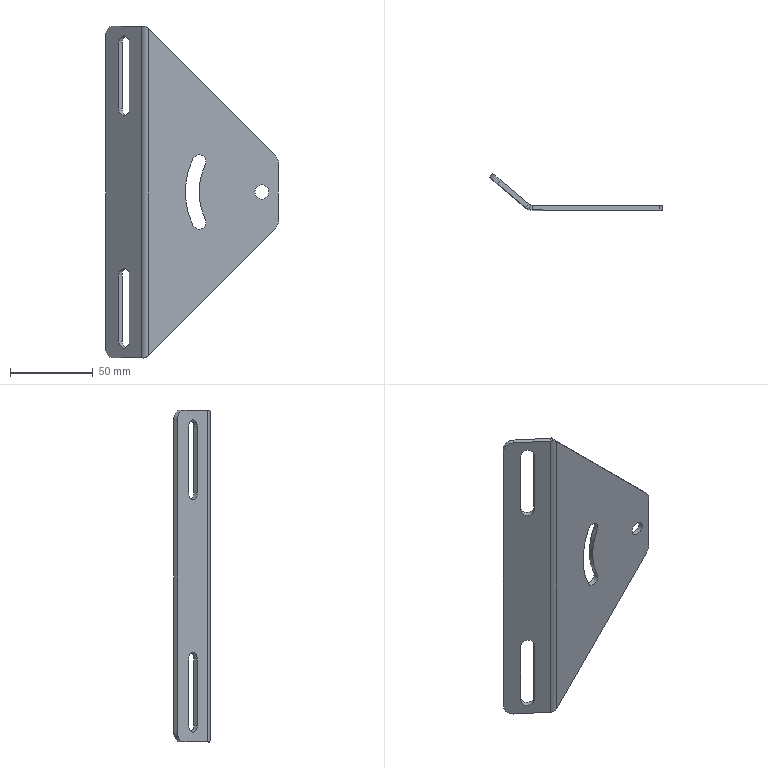Part | STEP file | Mounting leg part1 | 1 solid | 33 faces | box 104.175 x 22.016 x 200 mm | volume 43311 mm3 | plane 16 | cylinder 15 | spline 2 | commonest cylinder face diameters 12 x5 8.067 x2 8.131 x2 8.2 x2 6 x1 8.5 x1